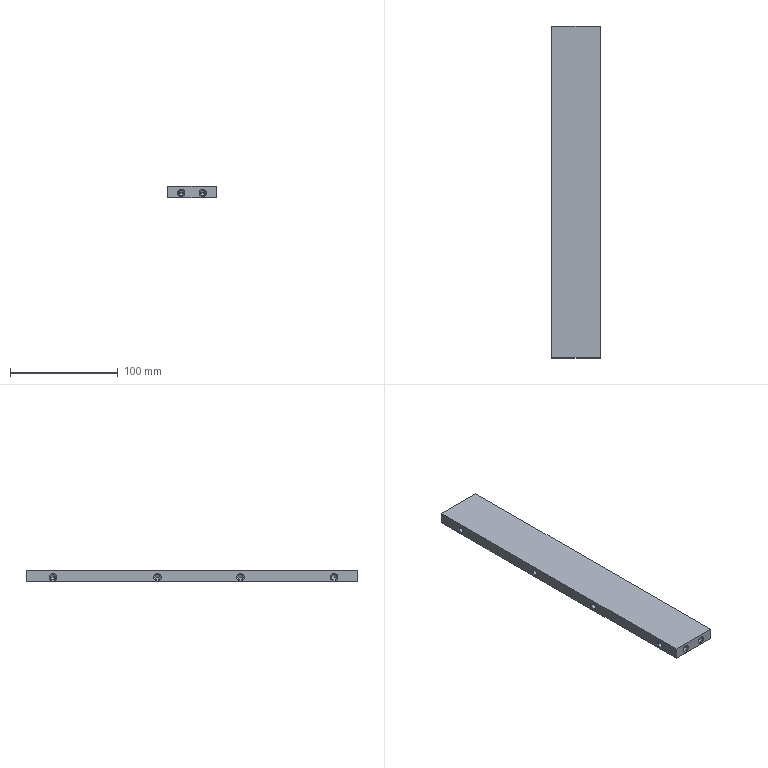Part | NX | 1 solid | 66 faces | box 45 x 308 x 10.5 mm | volume 142048 mm3 | cone 40 | cylinder 20 | plane 6 | commonest cylinder face diameters 5 x20